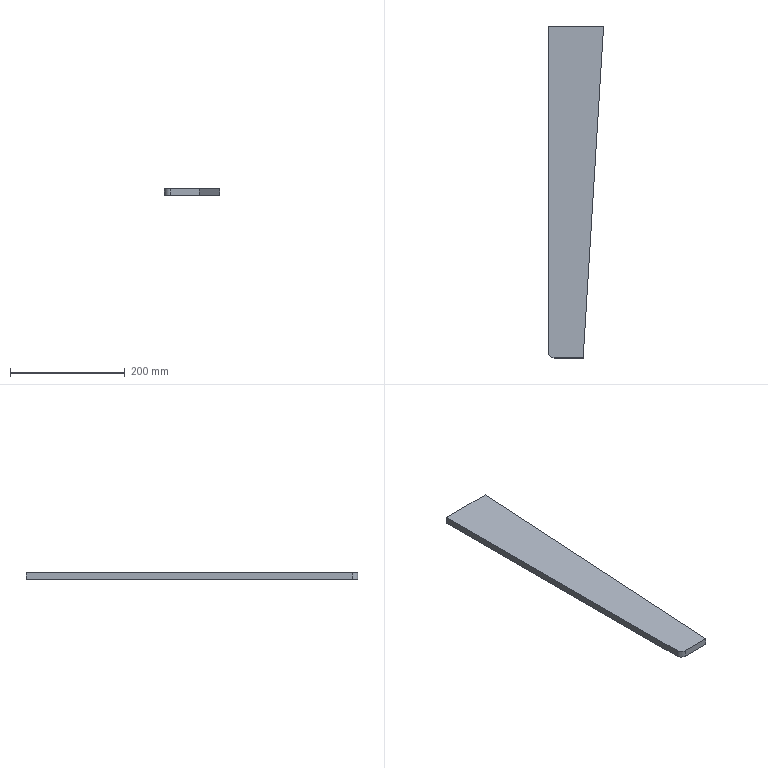Part | SolidWorks | features Extrusion 1 | 1 solid | 7 faces | box 96 x 578 x 12 mm | volume 542484 mm3 | plane 6 | cylinder 1 | commonest cylinder face diameters 20 x1
STEP:
#1=CARTESIAN_POINT('',(96.,578.,0.));
#2=VERTEX_POINT('',#1);
#3=CARTESIAN_POINT('',(0.,578.,0.));
#4=VERTEX_POINT('',#3);
#5=CARTESIAN_POINT('',(0.,578.,0.));
#6=DIRECTION('',(-1.,0.,0.));
#7=VECTOR('',#6,1000.);
#8=LINE('',#5,#7);
#9=EDGE_CURVE('',#2,#4,#8,.T.);
#10=ORIENTED_EDGE('',*,*,#9,.T.);
#11=CARTESIAN_POINT('',(0.,578.,12.));
#12=VERTEX_POINT('',#11);
#13=CARTESIAN_POINT('',(0.,578.,12.));
#14=DIRECTION('',(0.,0.,-1.));
#15=VECTOR('',#14,1000.);
#16=LINE('',#13,#15);
#17=EDGE_CURVE('',#12,#4,#16,.T.);
#18=ORIENTED_EDGE('',*,*,#17,.F.);
#19=CARTESIAN_POINT('',(96.,578.,12.));
#20=VERTEX_POINT('',#19);
#21=CARTESIAN_POINT('',(0.,578.,12.));
#22=DIRECTION('',(-1.,0.,0.));
#23=VECTOR('',#22,1000.);
#24=LINE('',#21,#23);
#25=EDGE_CURVE('',#20,#12,#24,.T.);
#26=ORIENTED_EDGE('',*,*,#25,.F.);
#27=CARTESIAN_POINT('',(96.,578.,12.));
#28=DIRECTION('',(0.,0.,-1.));
#29=VECTOR('',#28,1000.);
#30=LINE('',#27,#29);
#31=EDGE_CURVE('',#20,#2,#30,.T.);
#32=ORIENTED_EDGE('',*,*,#31,.T.);
#33=EDGE_LOOP('',(#10,#18,#26,#32));
#34=FACE_OUTER_BOUND('',#33,.T.);
#35=CARTESIAN_POINT('',(0.,578.,12.));
#36=DIRECTION('',(0.,-1.,0.));
#37=DIRECTION('',(0.,0.,-1.));
#38=AXIS2_PLACEMENT_3D('',#35,#36,#37);
#39=PLANE('',#38);
#40=ADVANCED_FACE('',(#34),#39,.F.);
#41=CARTESIAN_POINT('',(0.,10.,0.));
#42=VERTEX_POINT('',#41);
#43=CARTESIAN_POINT('',(0.,10.,0.));
#44=DIRECTION('',(0.,-1.,0.));
#45=VECTOR('',#44,1000.);
#46=LINE('',#43,#45);
#47=EDGE_CURVE('',#4,#42,#46,.T.);
#48=ORIENTED_EDGE('',*,*,#47,.T.);
#49=CARTESIAN_POINT('',(0.,10.,12.));
#50=VERTEX_POINT('',#49);
#51=CARTESIAN_POINT('',(0.,10.,12.));
#52=DIRECTION('',(0.,0.,-1.));
#53=VECTOR('',#52,1000.);
#54=LINE('',#51,#53);
#55=EDGE_CURVE('',#50,#42,#54,.T.);
#56=ORIENTED_EDGE('',*,*,#55,.F.);
#57=CARTESIAN_POINT('',(0.,10.,12.));
#58=DIRECTION('',(0.,-1.,0.));
#59=VECTOR('',#58,1000.);
#60=LINE('',#57,#59);
#61=EDGE_CURVE('',#12,#50,#60,.T.);
#62=ORIENTED_EDGE('',*,*,#61,.F.);
#63=ORIENTED_EDGE('',*,*,#17,.T.);
#64=EDGE_LOOP('',(#48,#56,#62,#63));
#65=FACE_OUTER_BOUND('',#64,.T.);
#66=CARTESIAN_POINT('',(0.,10.,12.));
#67=DIRECTION('',(1.,0.,0.));
#68=DIRECTION('',(0.,0.,-1.));
#69=AXIS2_PLACEMENT_3D('',#66,#67,#68);
#70=PLANE('',#69);
#71=ADVANCED_FACE('',(#65),#70,.F.);
#72=CARTESIAN_POINT('',(10.,0.,0.));
#73=VERTEX_POINT('',#72);
#74=CARTESIAN_POINT('',(10.,10.,0.));
#75=DIRECTION('',(0.,0.,1.));
#76=DIRECTION('',(1.,0.,0.));
#77=AXIS2_PLACEMENT_3D('',#74,#75,#76);
#78=CIRCLE('',#77,10.);
#79=EDGE_CURVE('',#42,#73,#78,.T.);
#80=ORIENTED_EDGE('',*,*,#79,.T.);
#81=CARTESIAN_POINT('',(10.,0.,12.));
#82=VERTEX_POINT('',#81);
#83=CARTESIAN_POINT('',(10.,0.,12.));
#84=DIRECTION('',(0.,0.,-1.));
#85=VECTOR('',#84,1000.);
#86=LINE('',#83,#85);
#87=EDGE_CURVE('',#82,#73,#86,.T.);
#88=ORIENTED_EDGE('',*,*,#87,.F.);
#89=CARTESIAN_POINT('',(10.,10.,12.));
#90=DIRECTION('',(0.,0.,1.));
#91=DIRECTION('',(1.,0.,0.));
#92=AXIS2_PLACEMENT_3D('',#89,#90,#91);
#93=CIRCLE('',#92,10.);
#94=EDGE_CURVE('',#50,#82,#93,.T.);
#95=ORIENTED_EDGE('',*,*,#94,.F.);
#96=ORIENTED_EDGE('',*,*,#55,.T.);
#97=EDGE_LOOP('',(#80,#88,#95,#96));
#98=FACE_OUTER_BOUND('',#97,.T.);
#99=CARTESIAN_POINT('',(10.,10.,12.));
#100=DIRECTION('',(0.,0.,-1.));
#101=DIRECTION('',(-1.,0.,0.));
#102=AXIS2_PLACEMENT_3D('',#99,#100,#101);
#103=CYLINDRICAL_SURFACE('',#102,10.);
#104=ADVANCED_FACE('',(#98),#103,.T.);
#105=CARTESIAN_POINT('',(60.5,0.,0.));
#106=VERTEX_POINT('',#105);
#107=CARTESIAN_POINT('',(60.5,0.,0.));
#108=DIRECTION('',(1.,0.,0.));
#109=VECTOR('',#108,1000.);
#110=LINE('',#107,#109);
#111=EDGE_CURVE('',#73,#106,#110,.T.);
#112=ORIENTED_EDGE('',*,*,#111,.T.);
#113=CARTESIAN_POINT('',(60.5,0.,12.));
#114=VERTEX_POINT('',#113);
#115=CARTESIAN_POINT('',(60.5,0.,12.));
#116=DIRECTION('',(0.,0.,-1.));
#117=VECTOR('',#116,1000.);
#118=LINE('',#115,#117);
#119=EDGE_CURVE('',#114,#106,#118,.T.);
#120=ORIENTED_EDGE('',*,*,#119,.F.);
#121=CARTESIAN_POINT('',(60.5,0.,12.));
#122=DIRECTION('',(1.,0.,0.));
#123=VECTOR('',#122,1000.);
#124=LINE('',#121,#123);
#125=EDGE_CURVE('',#82,#114,#124,.T.);
#126=ORIENTED_EDGE('',*,*,#125,.F.);
#127=ORIENTED_EDGE('',*,*,#87,.T.);
#128=EDGE_LOOP('',(#112,#120,#126,#127));
#129=FACE_OUTER_BOUND('',#128,.T.);
#130=CARTESIAN_POINT('',(60.5,0.,12.));
#131=DIRECTION('',(0.,1.,0.));
#132=DIRECTION('',(-1.,0.,0.));
#133=AXIS2_PLACEMENT_3D('',#130,#131,#132);
#134=PLANE('',#133);
#135=ADVANCED_FACE('',(#129),#134,.F.);
#136=CARTESIAN_POINT('',(96.,578.,0.));
#137=DIRECTION('',(0.0613,0.9981,0.));
#138=VECTOR('',#137,1000.);
#139=LINE('',#136,#138);
#140=EDGE_CURVE('',#106,#2,#139,.T.);
#141=ORIENTED_EDGE('',*,*,#140,.T.);
#142=ORIENTED_EDGE('',*,*,#31,.F.);
#143=CARTESIAN_POINT('',(96.,578.,12.));
#144=DIRECTION('',(0.0613,0.9981,0.));
#145=VECTOR('',#144,1000.);
#146=LINE('',#143,#145);
#147=EDGE_CURVE('',#114,#20,#146,.T.);
#148=ORIENTED_EDGE('',*,*,#147,.F.);
#149=ORIENTED_EDGE('',*,*,#119,.T.);
#150=EDGE_LOOP('',(#141,#142,#148,#149));
#151=FACE_OUTER_BOUND('',#150,.T.);
#152=CARTESIAN_POINT('',(96.,578.,12.));
#153=DIRECTION('',(-0.9981,0.0613,0.));
#154=DIRECTION('',(-0.0613,-0.9981,0.));
#155=AXIS2_PLACEMENT_3D('',#152,#153,#154);
#156=PLANE('',#155);
#157=ADVANCED_FACE('',(#151),#156,.F.);
#158=ORIENTED_EDGE('',*,*,#25,.T.);
#159=ORIENTED_EDGE('',*,*,#61,.T.);
#160=ORIENTED_EDGE('',*,*,#94,.T.);
#161=ORIENTED_EDGE('',*,*,#125,.T.);
#162=ORIENTED_EDGE('',*,*,#147,.T.);
#163=EDGE_LOOP('',(#158,#159,#160,#161,#162));
#164=FACE_OUTER_BOUND('',#163,.T.);
#165=CARTESIAN_POINT('',(10.,10.,12.));
#166=DIRECTION('',(0.,0.,1.));
#167=DIRECTION('',(1.,0.,0.));
#168=AXIS2_PLACEMENT_3D('',#165,#166,#167);
#169=PLANE('',#168);
#170=ADVANCED_FACE('',(#164),#169,.T.);
#171=ORIENTED_EDGE('',*,*,#9,.F.);
#172=ORIENTED_EDGE('',*,*,#140,.F.);
#173=ORIENTED_EDGE('',*,*,#111,.F.);
#174=ORIENTED_EDGE('',*,*,#79,.F.);
#175=ORIENTED_EDGE('',*,*,#47,.F.);
#176=EDGE_LOOP('',(#171,#172,#173,#174,#175));
#177=FACE_OUTER_BOUND('',#176,.T.);
#178=CARTESIAN_POINT('',(10.,10.,0.));
#179=DIRECTION('',(0.,0.,1.));
#180=DIRECTION('',(1.,0.,0.));
#181=AXIS2_PLACEMENT_3D('',#178,#179,#180);
#182=PLANE('',#181);
#183=ADVANCED_FACE('',(#177),#182,.F.);
#184=CLOSED_SHELL('',(#40,#71,#104,#135,#157,#170,#183));
#185=MANIFOLD_SOLID_BREP('',#184);
#186=CARTESIAN_POINT('',(0.,0.,0.));
#187=DIRECTION('',(0.,0.,1.));
#188=DIRECTION('',(1.,0.,0.));
#189=AXIS2_PLACEMENT_3D('',#186,#187,#188);
#190=(LENGTH_UNIT()NAMED_UNIT(*)SI_UNIT(.MILLI.,.METRE.));
#191=UNCERTAINTY_MEASURE_WITH_UNIT(LENGTH_MEASURE(0.00001),#190,'','');
#192=(NAMED_UNIT(*)PLANE_ANGLE_UNIT()SI_UNIT($,.RADIAN.));
#193=(NAMED_UNIT(*)SI_UNIT($,.STERADIAN.)SOLID_ANGLE_UNIT());
#194=(GEOMETRIC_REPRESENTATION_CONTEXT(3)GLOBAL_UNCERTAINTY_ASSIGNED_CONTEXT((#191))GLOBAL_UNIT_ASSIGNED_CONTEXT((#190,#192,#193))REPRESENTATION_CONTEXT('',''));
#195=ADVANCED_BREP_SHAPE_REPRESENTATION('',(#185,#189),#194);